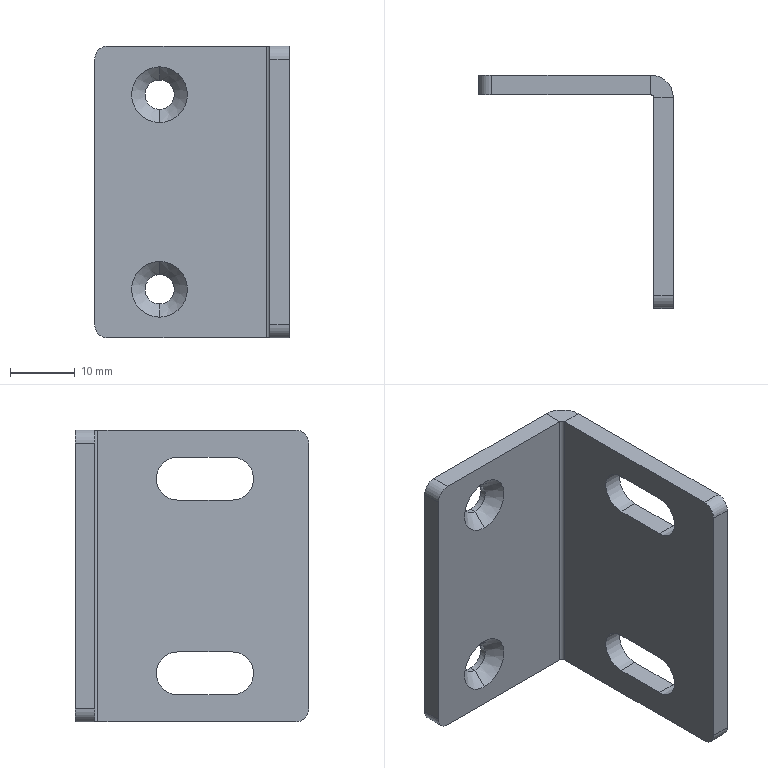Part | STEP file | Tabletop mounting plate A | 1 solid | 34 faces | box 30 x 36 x 45 mm | volume 7668 mm3 | plane 16 | cylinder 14 | cone 4 | commonest cylinder face diameters 4 x4 4.5 x4 6.6 x4 1 x1 7 x1